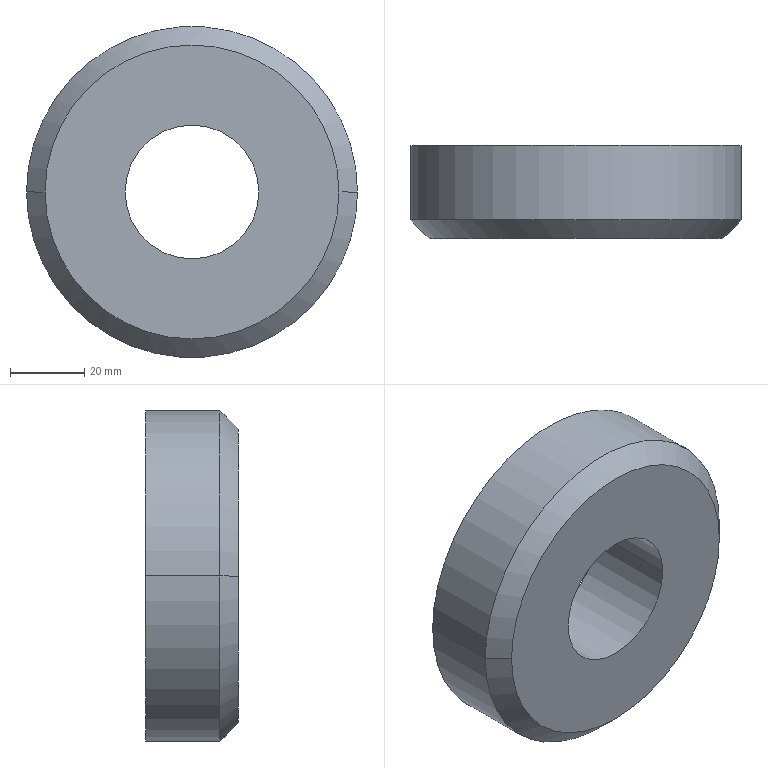Part | SolidWorks | features Chamfer 1, Revolution 1 | 1 solid | 8 faces | box 89 x 25 x 89 mm | volume 126717 mm3 | cylinder 4 | cone 2 | plane 2 | commonest cylinder face diameters 36 x2 89 x2
STEP:
#1=CARTESIAN_POINT('',(39.5,0.,0.));
#2=VERTEX_POINT('',#1);
#3=CARTESIAN_POINT('',(-39.5,0.,0.));
#4=VERTEX_POINT('',#3);
#5=CARTESIAN_POINT('',(0.,0.,0.));
#6=DIRECTION('',(0.,-1.,0.));
#7=DIRECTION('',(1.,0.,0.));
#8=AXIS2_PLACEMENT_3D('',#5,#6,#7);
#9=CIRCLE('',#8,39.5);
#10=EDGE_CURVE('',#2,#4,#9,.T.);
#11=ORIENTED_EDGE('',*,*,#10,.F.);
#12=CARTESIAN_POINT('',(44.5,5.,0.));
#13=VERTEX_POINT('',#12);
#14=CARTESIAN_POINT('',(39.5,0.,0.));
#15=DIRECTION('',(0.7071,0.7071,0.));
#16=VECTOR('',#15,1000.);
#17=LINE('',#14,#16);
#18=EDGE_CURVE('',#2,#13,#17,.T.);
#19=ORIENTED_EDGE('',*,*,#18,.T.);
#20=CARTESIAN_POINT('',(-44.5,5.,0.));
#21=VERTEX_POINT('',#20);
#22=CARTESIAN_POINT('',(0.,5.,0.));
#23=DIRECTION('',(0.,1.,0.));
#24=DIRECTION('',(1.,0.,0.));
#25=AXIS2_PLACEMENT_3D('',#22,#23,#24);
#26=CIRCLE('',#25,44.5);
#27=EDGE_CURVE('',#21,#13,#26,.T.);
#28=ORIENTED_EDGE('',*,*,#27,.F.);
#29=CARTESIAN_POINT('',(-39.5,0.,0.));
#30=DIRECTION('',(-0.7071,0.7071,0.));
#31=VECTOR('',#30,1000.);
#32=LINE('',#29,#31);
#33=EDGE_CURVE('',#4,#21,#32,.T.);
#34=ORIENTED_EDGE('',*,*,#33,.F.);
#35=EDGE_LOOP('',(#11,#19,#28,#34));
#36=FACE_OUTER_BOUND('',#35,.T.);
#37=CARTESIAN_POINT('',(0.,0.,0.));
#38=DIRECTION('',(0.,1.,0.));
#39=DIRECTION('',(-1.,0.,0.));
#40=AXIS2_PLACEMENT_3D('',#37,#38,#39);
#41=CONICAL_SURFACE('',#40,39.5,0.7854);
#42=ADVANCED_FACE('',(#36),#41,.T.);
#43=CARTESIAN_POINT('',(44.5,25.,0.));
#44=VERTEX_POINT('',#43);
#45=CARTESIAN_POINT('',(-44.5,25.,0.));
#46=VERTEX_POINT('',#45);
#47=CARTESIAN_POINT('',(0.,25.,0.));
#48=DIRECTION('',(0.,-1.,0.));
#49=DIRECTION('',(1.,0.,0.));
#50=AXIS2_PLACEMENT_3D('',#47,#48,#49);
#51=CIRCLE('',#50,44.5);
#52=EDGE_CURVE('',#44,#46,#51,.T.);
#53=ORIENTED_EDGE('',*,*,#52,.T.);
#54=CARTESIAN_POINT('',(-44.5,-964.354,0.));
#55=DIRECTION('',(0.,-1.,0.));
#56=VECTOR('',#55,1000.);
#57=LINE('',#54,#56);
#58=EDGE_CURVE('',#46,#21,#57,.T.);
#59=ORIENTED_EDGE('',*,*,#58,.T.);
#60=ORIENTED_EDGE('',*,*,#27,.T.);
#61=CARTESIAN_POINT('',(44.5,-964.354,0.));
#62=DIRECTION('',(0.,-1.,0.));
#63=VECTOR('',#62,1000.);
#64=LINE('',#61,#63);
#65=EDGE_CURVE('',#44,#13,#64,.T.);
#66=ORIENTED_EDGE('',*,*,#65,.F.);
#67=EDGE_LOOP('',(#53,#59,#60,#66));
#68=FACE_OUTER_BOUND('',#67,.T.);
#69=CARTESIAN_POINT('',(0.,-964.354,0.));
#70=DIRECTION('',(0.,-1.,0.));
#71=DIRECTION('',(1.,0.,0.));
#72=AXIS2_PLACEMENT_3D('',#69,#70,#71);
#73=CYLINDRICAL_SURFACE('',#72,44.5);
#74=ADVANCED_FACE('',(#68),#73,.T.);
#75=CARTESIAN_POINT('',(-18.,25.,0.));
#76=VERTEX_POINT('',#75);
#77=CARTESIAN_POINT('',(18.,25.,0.));
#78=VERTEX_POINT('',#77);
#79=CARTESIAN_POINT('',(0.,25.,0.));
#80=DIRECTION('',(0.,-1.,0.));
#81=DIRECTION('',(1.,0.,0.));
#82=AXIS2_PLACEMENT_3D('',#79,#80,#81);
#83=CIRCLE('',#82,18.);
#84=EDGE_CURVE('',#76,#78,#83,.T.);
#85=ORIENTED_EDGE('',*,*,#84,.F.);
#86=CARTESIAN_POINT('',(-18.,0.,0.));
#87=VERTEX_POINT('',#86);
#88=CARTESIAN_POINT('',(-18.,-964.354,0.));
#89=DIRECTION('',(0.,-1.,0.));
#90=VECTOR('',#89,1000.);
#91=LINE('',#88,#90);
#92=EDGE_CURVE('',#76,#87,#91,.T.);
#93=ORIENTED_EDGE('',*,*,#92,.T.);
#94=CARTESIAN_POINT('',(18.,0.,0.));
#95=VERTEX_POINT('',#94);
#96=CARTESIAN_POINT('',(0.,0.,0.));
#97=DIRECTION('',(0.,-1.,0.));
#98=DIRECTION('',(1.,0.,0.));
#99=AXIS2_PLACEMENT_3D('',#96,#97,#98);
#100=CIRCLE('',#99,18.);
#101=EDGE_CURVE('',#87,#95,#100,.T.);
#102=ORIENTED_EDGE('',*,*,#101,.T.);
#103=CARTESIAN_POINT('',(18.,-964.354,0.));
#104=DIRECTION('',(0.,-1.,0.));
#105=VECTOR('',#104,1000.);
#106=LINE('',#103,#105);
#107=EDGE_CURVE('',#78,#95,#106,.T.);
#108=ORIENTED_EDGE('',*,*,#107,.F.);
#109=EDGE_LOOP('',(#85,#93,#102,#108));
#110=FACE_OUTER_BOUND('',#109,.T.);
#111=CARTESIAN_POINT('',(0.,-964.354,0.));
#112=DIRECTION('',(0.,-1.,0.));
#113=DIRECTION('',(1.,0.,0.));
#114=AXIS2_PLACEMENT_3D('',#111,#112,#113);
#115=CYLINDRICAL_SURFACE('',#114,18.);
#116=ADVANCED_FACE('',(#110),#115,.F.);
#117=ORIENTED_EDGE('',*,*,#92,.F.);
#118=CARTESIAN_POINT('',(0.,25.,0.));
#119=DIRECTION('',(0.,-1.,0.));
#120=DIRECTION('',(1.,0.,0.));
#121=AXIS2_PLACEMENT_3D('',#118,#119,#120);
#122=CIRCLE('',#121,18.);
#123=EDGE_CURVE('',#78,#76,#122,.T.);
#124=ORIENTED_EDGE('',*,*,#123,.F.);
#125=ORIENTED_EDGE('',*,*,#107,.T.);
#126=CARTESIAN_POINT('',(0.,0.,0.));
#127=DIRECTION('',(0.,-1.,0.));
#128=DIRECTION('',(1.,0.,0.));
#129=AXIS2_PLACEMENT_3D('',#126,#127,#128);
#130=CIRCLE('',#129,18.);
#131=EDGE_CURVE('',#95,#87,#130,.T.);
#132=ORIENTED_EDGE('',*,*,#131,.T.);
#133=EDGE_LOOP('',(#117,#124,#125,#132));
#134=FACE_OUTER_BOUND('',#133,.T.);
#135=CARTESIAN_POINT('',(0.,-964.354,0.));
#136=DIRECTION('',(0.,-1.,0.));
#137=DIRECTION('',(1.,0.,0.));
#138=AXIS2_PLACEMENT_3D('',#135,#136,#137);
#139=CYLINDRICAL_SURFACE('',#138,18.);
#140=ADVANCED_FACE('',(#134),#139,.F.);
#141=ORIENTED_EDGE('',*,*,#123,.T.);
#142=ORIENTED_EDGE('',*,*,#84,.T.);
#143=EDGE_LOOP('',(#141,#142));
#144=FACE_BOUND('',#143,.T.);
#145=ORIENTED_EDGE('',*,*,#52,.F.);
#146=CARTESIAN_POINT('',(0.,25.,0.));
#147=DIRECTION('',(0.,-1.,0.));
#148=DIRECTION('',(1.,0.,0.));
#149=AXIS2_PLACEMENT_3D('',#146,#147,#148);
#150=CIRCLE('',#149,44.5);
#151=EDGE_CURVE('',#46,#44,#150,.T.);
#152=ORIENTED_EDGE('',*,*,#151,.F.);
#153=EDGE_LOOP('',(#145,#152));
#154=FACE_OUTER_BOUND('',#153,.T.);
#155=CARTESIAN_POINT('',(18.,25.,0.));
#156=DIRECTION('',(0.,1.,0.));
#157=DIRECTION('',(-1.,0.,0.));
#158=AXIS2_PLACEMENT_3D('',#155,#156,#157);
#159=PLANE('',#158);
#160=ADVANCED_FACE('',(#144,#154),#159,.T.);
#161=ORIENTED_EDGE('',*,*,#58,.F.);
#162=ORIENTED_EDGE('',*,*,#151,.T.);
#163=ORIENTED_EDGE('',*,*,#65,.T.);
#164=CARTESIAN_POINT('',(0.,5.,0.));
#165=DIRECTION('',(0.,1.,0.));
#166=DIRECTION('',(1.,0.,0.));
#167=AXIS2_PLACEMENT_3D('',#164,#165,#166);
#168=CIRCLE('',#167,44.5);
#169=EDGE_CURVE('',#13,#21,#168,.T.);
#170=ORIENTED_EDGE('',*,*,#169,.T.);
#171=EDGE_LOOP('',(#161,#162,#163,#170));
#172=FACE_OUTER_BOUND('',#171,.T.);
#173=CARTESIAN_POINT('',(0.,-964.354,0.));
#174=DIRECTION('',(0.,-1.,0.));
#175=DIRECTION('',(1.,0.,0.));
#176=AXIS2_PLACEMENT_3D('',#173,#174,#175);
#177=CYLINDRICAL_SURFACE('',#176,44.5);
#178=ADVANCED_FACE('',(#172),#177,.T.);
#179=CARTESIAN_POINT('',(0.,0.,0.));
#180=DIRECTION('',(0.,-1.,0.));
#181=DIRECTION('',(1.,0.,0.));
#182=AXIS2_PLACEMENT_3D('',#179,#180,#181);
#183=CIRCLE('',#182,39.5);
#184=EDGE_CURVE('',#4,#2,#183,.T.);
#185=ORIENTED_EDGE('',*,*,#184,.T.);
#186=ORIENTED_EDGE('',*,*,#10,.T.);
#187=EDGE_LOOP('',(#185,#186));
#188=FACE_OUTER_BOUND('',#187,.T.);
#189=ORIENTED_EDGE('',*,*,#131,.F.);
#190=ORIENTED_EDGE('',*,*,#101,.F.);
#191=EDGE_LOOP('',(#189,#190));
#192=FACE_BOUND('',#191,.T.);
#193=CARTESIAN_POINT('',(18.,0.,0.));
#194=DIRECTION('',(0.,-1.,0.));
#195=DIRECTION('',(1.,0.,0.));
#196=AXIS2_PLACEMENT_3D('',#193,#194,#195);
#197=PLANE('',#196);
#198=ADVANCED_FACE('',(#188,#192),#197,.T.);
#199=ORIENTED_EDGE('',*,*,#18,.F.);
#200=ORIENTED_EDGE('',*,*,#184,.F.);
#201=ORIENTED_EDGE('',*,*,#33,.T.);
#202=ORIENTED_EDGE('',*,*,#169,.F.);
#203=EDGE_LOOP('',(#199,#200,#201,#202));
#204=FACE_OUTER_BOUND('',#203,.T.);
#205=CARTESIAN_POINT('',(0.,0.,0.));
#206=DIRECTION('',(0.,1.,0.));
#207=DIRECTION('',(-1.,0.,0.));
#208=AXIS2_PLACEMENT_3D('',#205,#206,#207);
#209=CONICAL_SURFACE('',#208,39.5,0.7854);
#210=ADVANCED_FACE('',(#204),#209,.T.);
#211=CLOSED_SHELL('',(#42,#74,#116,#140,#160,#178,#198,#210));
#212=MANIFOLD_SOLID_BREP('',#211);
#213=CARTESIAN_POINT('',(0.,0.,0.));
#214=DIRECTION('',(0.,0.,1.));
#215=DIRECTION('',(1.,0.,0.));
#216=AXIS2_PLACEMENT_3D('',#213,#214,#215);
#217=(LENGTH_UNIT()NAMED_UNIT(*)SI_UNIT(.MILLI.,.METRE.));
#218=UNCERTAINTY_MEASURE_WITH_UNIT(LENGTH_MEASURE(0.00001),#217,'','');
#219=(NAMED_UNIT(*)PLANE_ANGLE_UNIT()SI_UNIT($,.RADIAN.));
#220=(NAMED_UNIT(*)SI_UNIT($,.STERADIAN.)SOLID_ANGLE_UNIT());
#221=(GEOMETRIC_REPRESENTATION_CONTEXT(3)GLOBAL_UNCERTAINTY_ASSIGNED_CONTEXT((#218))GLOBAL_UNIT_ASSIGNED_CONTEXT((#217,#219,#220))REPRESENTATION_CONTEXT('',''));
#222=ADVANCED_BREP_SHAPE_REPRESENTATION('',(#212,#216),#221);